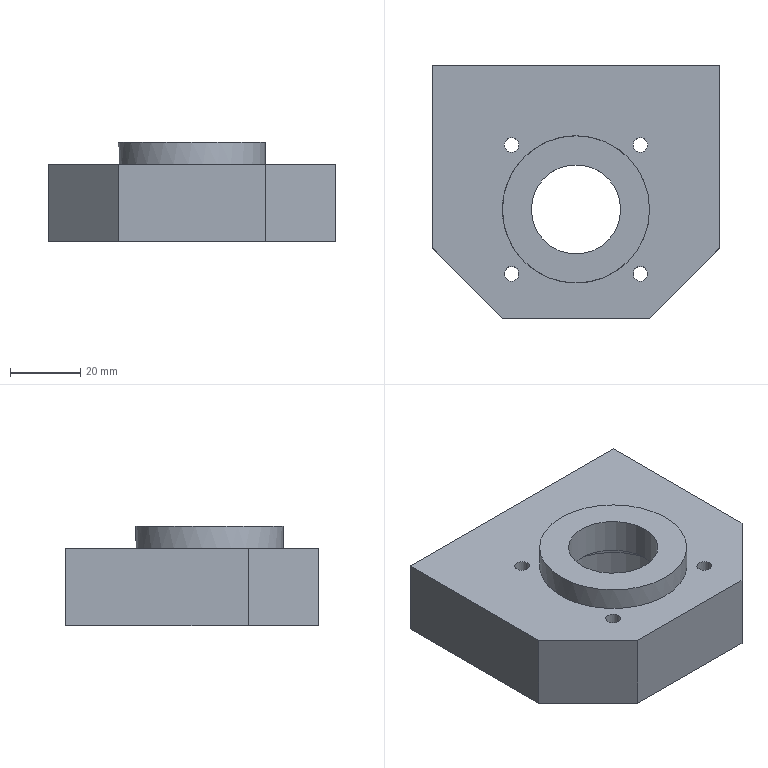Part | NX | features EXTRUDE 7, DATUM_CSYS 2, SKETCH 2, LINKED_FACE 1 | 1 solid | 23 faces | box 82 x 72 x 28.5 mm | volume 96953 mm3 | plane 13 | cylinder 10 | commonest cylinder face diameters 4.2 x4 8.5 x2 42 x2 25.5 x1 36 x1
STEP:
#1=CARTESIAN_POINT('',(-18.,0.,3.));
#2=VERTEX_POINT('',#1);
#3=CARTESIAN_POINT('',(0.,0.,3.));
#4=DIRECTION('',(0.,0.,1.));
#5=DIRECTION('',(-1.,0.,0.));
#6=AXIS2_PLACEMENT_3D('',#3,#4,#5);
#7=CIRCLE('',#6,18.);
#8=EDGE_CURVE('',#2,#2,#7,.T.);
#9=ORIENTED_EDGE('',*,*,#8,.F.);
#10=EDGE_LOOP('',(#9));
#11=FACE_BOUND('',#10,.T.);
#12=CARTESIAN_POINT('',(18.,0.,7.5));
#13=VERTEX_POINT('',#12);
#14=CARTESIAN_POINT('',(0.,0.,7.5));
#15=DIRECTION('',(0.,0.,-1.));
#16=DIRECTION('',(1.,0.,0.));
#17=AXIS2_PLACEMENT_3D('',#14,#15,#16);
#18=CIRCLE('',#17,18.);
#19=EDGE_CURVE('',#13,#13,#18,.T.);
#20=ORIENTED_EDGE('',*,*,#19,.F.);
#21=EDGE_LOOP('',(#20));
#22=FACE_BOUND('',#21,.T.);
#23=CARTESIAN_POINT('',(0.,0.,3.));
#24=DIRECTION('',(0.,0.,1.));
#25=DIRECTION('',(1.,0.,0.));
#26=AXIS2_PLACEMENT_3D('',#23,#24,#25);
#27=CYLINDRICAL_SURFACE('',#26,18.);
#28=ADVANCED_FACE('',(#11,#22),#27,.F.);
#29=CARTESIAN_POINT('',(21.,0.,-11.));
#30=VERTEX_POINT('',#29);
#31=CARTESIAN_POINT('',(0.,0.,-11.));
#32=DIRECTION('',(0.,0.,1.));
#33=DIRECTION('',(1.,0.,0.));
#34=AXIS2_PLACEMENT_3D('',#31,#32,#33);
#35=CIRCLE('',#34,21.);
#36=EDGE_CURVE('',#30,#30,#35,.F.);
#37=ORIENTED_EDGE('',*,*,#36,.T.);
#38=EDGE_LOOP('',(#37));
#39=FACE_BOUND('',#38,.T.);
#40=CARTESIAN_POINT('',(21.,0.,3.));
#41=VERTEX_POINT('',#40);
#42=CARTESIAN_POINT('',(0.,0.,3.));
#43=DIRECTION('',(0.,0.,1.));
#44=DIRECTION('',(1.,0.,0.));
#45=AXIS2_PLACEMENT_3D('',#42,#43,#44);
#46=CIRCLE('',#45,21.);
#47=EDGE_CURVE('',#41,#41,#46,.T.);
#48=ORIENTED_EDGE('',*,*,#47,.T.);
#49=EDGE_LOOP('',(#48));
#50=FACE_BOUND('',#49,.T.);
#51=CARTESIAN_POINT('',(0.,0.,9.));
#52=DIRECTION('',(0.,0.,-1.));
#53=DIRECTION('',(-1.,0.,0.));
#54=AXIS2_PLACEMENT_3D('',#51,#52,#53);
#55=CYLINDRICAL_SURFACE('',#54,21.);
#56=ADVANCED_FACE('',(#39,#50),#55,.F.);
#57=CARTESIAN_POINT('',(41.,-11.,-11.));
#58=VERTEX_POINT('',#57);
#59=CARTESIAN_POINT('',(41.,41.,-11.));
#60=VERTEX_POINT('',#59);
#61=CARTESIAN_POINT('',(41.,-11.,-11.));
#62=DIRECTION('',(0.,1.,0.));
#63=VECTOR('',#62,1000.);
#64=LINE('',#61,#63);
#65=EDGE_CURVE('',#58,#60,#64,.T.);
#66=ORIENTED_EDGE('',*,*,#65,.T.);
#67=CARTESIAN_POINT('',(41.,41.,11.));
#68=VERTEX_POINT('',#67);
#69=CARTESIAN_POINT('',(41.,41.,11.));
#70=DIRECTION('',(0.,0.,-1.));
#71=VECTOR('',#70,1000.);
#72=LINE('',#69,#71);
#73=EDGE_CURVE('',#68,#60,#72,.T.);
#74=ORIENTED_EDGE('',*,*,#73,.F.);
#75=CARTESIAN_POINT('',(41.,-11.,11.));
#76=VERTEX_POINT('',#75);
#77=CARTESIAN_POINT('',(41.,-11.,11.));
#78=DIRECTION('',(0.,1.,0.));
#79=VECTOR('',#78,1000.);
#80=LINE('',#77,#79);
#81=EDGE_CURVE('',#76,#68,#80,.T.);
#82=ORIENTED_EDGE('',*,*,#81,.F.);
#83=CARTESIAN_POINT('',(41.,-11.,11.));
#84=DIRECTION('',(0.,0.,-1.));
#85=VECTOR('',#84,1000.);
#86=LINE('',#83,#85);
#87=EDGE_CURVE('',#76,#58,#86,.T.);
#88=ORIENTED_EDGE('',*,*,#87,.T.);
#89=EDGE_LOOP('',(#66,#74,#82,#88));
#90=FACE_BOUND('',#89,.T.);
#91=CARTESIAN_POINT('',(41.,-11.,11.));
#92=DIRECTION('',(-1.,0.,0.));
#93=DIRECTION('',(0.,0.,1.));
#94=AXIS2_PLACEMENT_3D('',#91,#92,#93);
#95=PLANE('',#94);
#96=ADVANCED_FACE('',(#90),#95,.F.);
#97=CARTESIAN_POINT('',(30.,41.,-4.25));
#98=VERTEX_POINT('',#97);
#99=CARTESIAN_POINT('',(30.,41.,0.));
#100=DIRECTION('',(0.,-1.,0.));
#101=DIRECTION('',(0.,0.,-1.));
#102=AXIS2_PLACEMENT_3D('',#99,#100,#101);
#103=CIRCLE('',#102,4.25);
#104=EDGE_CURVE('',#98,#98,#103,.T.);
#105=ORIENTED_EDGE('',*,*,#104,.T.);
#106=EDGE_LOOP('',(#105));
#107=FACE_BOUND('',#106,.T.);
#108=CARTESIAN_POINT('',(-30.,41.,-4.25));
#109=VERTEX_POINT('',#108);
#110=CARTESIAN_POINT('',(-30.,41.,0.));
#111=DIRECTION('',(0.,-1.,0.));
#112=DIRECTION('',(0.,0.,-1.));
#113=AXIS2_PLACEMENT_3D('',#110,#111,#112);
#114=CIRCLE('',#113,4.25);
#115=EDGE_CURVE('',#109,#109,#114,.T.);
#116=ORIENTED_EDGE('',*,*,#115,.T.);
#117=EDGE_LOOP('',(#116));
#118=FACE_BOUND('',#117,.T.);
#119=CARTESIAN_POINT('',(-41.,41.,-11.));
#120=VERTEX_POINT('',#119);
#121=CARTESIAN_POINT('',(41.,41.,-11.));
#122=DIRECTION('',(-1.,0.,0.));
#123=VECTOR('',#122,1000.);
#124=LINE('',#121,#123);
#125=EDGE_CURVE('',#60,#120,#124,.T.);
#126=ORIENTED_EDGE('',*,*,#125,.T.);
#127=CARTESIAN_POINT('',(-41.,41.,11.));
#128=VERTEX_POINT('',#127);
#129=CARTESIAN_POINT('',(-41.,41.,11.));
#130=DIRECTION('',(0.,0.,-1.));
#131=VECTOR('',#130,1000.);
#132=LINE('',#129,#131);
#133=EDGE_CURVE('',#128,#120,#132,.T.);
#134=ORIENTED_EDGE('',*,*,#133,.F.);
#135=CARTESIAN_POINT('',(41.,41.,11.));
#136=DIRECTION('',(-1.,0.,0.));
#137=VECTOR('',#136,1000.);
#138=LINE('',#135,#137);
#139=EDGE_CURVE('',#68,#128,#138,.T.);
#140=ORIENTED_EDGE('',*,*,#139,.F.);
#141=ORIENTED_EDGE('',*,*,#73,.T.);
#142=EDGE_LOOP('',(#126,#134,#140,#141));
#143=FACE_BOUND('',#142,.T.);
#144=CARTESIAN_POINT('',(41.,41.,11.));
#145=DIRECTION('',(0.,-1.,0.));
#146=DIRECTION('',(0.,0.,-1.));
#147=AXIS2_PLACEMENT_3D('',#144,#145,#146);
#148=PLANE('',#147);
#149=ADVANCED_FACE('',(#107,#118,#143),#148,.F.);
#150=CARTESIAN_POINT('',(-41.,-11.,-11.));
#151=VERTEX_POINT('',#150);
#152=CARTESIAN_POINT('',(-41.,41.,-11.));
#153=DIRECTION('',(0.,-1.,0.));
#154=VECTOR('',#153,1000.);
#155=LINE('',#152,#154);
#156=EDGE_CURVE('',#120,#151,#155,.T.);
#157=ORIENTED_EDGE('',*,*,#156,.T.);
#158=CARTESIAN_POINT('',(-41.,-11.,11.));
#159=VERTEX_POINT('',#158);
#160=CARTESIAN_POINT('',(-41.,-11.,11.));
#161=DIRECTION('',(0.,0.,-1.));
#162=VECTOR('',#161,1000.);
#163=LINE('',#160,#162);
#164=EDGE_CURVE('',#159,#151,#163,.T.);
#165=ORIENTED_EDGE('',*,*,#164,.F.);
#166=CARTESIAN_POINT('',(-41.,41.,11.));
#167=DIRECTION('',(0.,-1.,0.));
#168=VECTOR('',#167,1000.);
#169=LINE('',#166,#168);
#170=EDGE_CURVE('',#128,#159,#169,.T.);
#171=ORIENTED_EDGE('',*,*,#170,.F.);
#172=ORIENTED_EDGE('',*,*,#133,.T.);
#173=EDGE_LOOP('',(#157,#165,#171,#172));
#174=FACE_BOUND('',#173,.T.);
#175=CARTESIAN_POINT('',(-41.,41.,11.));
#176=DIRECTION('',(1.,0.,0.));
#177=DIRECTION('',(0.,0.,-1.));
#178=AXIS2_PLACEMENT_3D('',#175,#176,#177);
#179=PLANE('',#178);
#180=ADVANCED_FACE('',(#174),#179,.F.);
#181=CARTESIAN_POINT('',(-21.,-31.,-11.));
#182=VERTEX_POINT('',#181);
#183=CARTESIAN_POINT('',(-41.,-11.,-11.));
#184=DIRECTION('',(0.7071,-0.7071,0.));
#185=VECTOR('',#184,1000.);
#186=LINE('',#183,#185);
#187=EDGE_CURVE('',#151,#182,#186,.T.);
#188=ORIENTED_EDGE('',*,*,#187,.T.);
#189=CARTESIAN_POINT('',(-21.,-31.,11.));
#190=VERTEX_POINT('',#189);
#191=CARTESIAN_POINT('',(-21.,-31.,11.));
#192=DIRECTION('',(0.,0.,-1.));
#193=VECTOR('',#192,1000.);
#194=LINE('',#191,#193);
#195=EDGE_CURVE('',#190,#182,#194,.T.);
#196=ORIENTED_EDGE('',*,*,#195,.F.);
#197=CARTESIAN_POINT('',(-41.,-11.,11.));
#198=DIRECTION('',(0.7071,-0.7071,0.));
#199=VECTOR('',#198,1000.);
#200=LINE('',#197,#199);
#201=EDGE_CURVE('',#159,#190,#200,.T.);
#202=ORIENTED_EDGE('',*,*,#201,.F.);
#203=ORIENTED_EDGE('',*,*,#164,.T.);
#204=EDGE_LOOP('',(#188,#196,#202,#203));
#205=FACE_BOUND('',#204,.T.);
#206=CARTESIAN_POINT('',(-41.,-11.,11.));
#207=DIRECTION('',(0.7071,0.7071,0.));
#208=DIRECTION('',(-0.7071,0.7071,0.));
#209=AXIS2_PLACEMENT_3D('',#206,#207,#208);
#210=PLANE('',#209);
#211=ADVANCED_FACE('',(#205),#210,.F.);
#212=CARTESIAN_POINT('',(21.,-31.,-11.));
#213=VERTEX_POINT('',#212);
#214=CARTESIAN_POINT('',(-21.,-31.,-11.));
#215=DIRECTION('',(1.,0.,0.));
#216=VECTOR('',#215,1000.);
#217=LINE('',#214,#216);
#218=EDGE_CURVE('',#182,#213,#217,.T.);
#219=ORIENTED_EDGE('',*,*,#218,.T.);
#220=CARTESIAN_POINT('',(21.,-31.,11.));
#221=VERTEX_POINT('',#220);
#222=CARTESIAN_POINT('',(21.,-31.,11.));
#223=DIRECTION('',(0.,0.,-1.));
#224=VECTOR('',#223,1000.);
#225=LINE('',#222,#224);
#226=EDGE_CURVE('',#221,#213,#225,.T.);
#227=ORIENTED_EDGE('',*,*,#226,.F.);
#228=CARTESIAN_POINT('',(-21.,-31.,11.));
#229=DIRECTION('',(1.,0.,0.));
#230=VECTOR('',#229,1000.);
#231=LINE('',#228,#230);
#232=EDGE_CURVE('',#190,#221,#231,.T.);
#233=ORIENTED_EDGE('',*,*,#232,.F.);
#234=ORIENTED_EDGE('',*,*,#195,.T.);
#235=EDGE_LOOP('',(#219,#227,#233,#234));
#236=FACE_BOUND('',#235,.T.);
#237=CARTESIAN_POINT('',(-21.,-31.,11.));
#238=DIRECTION('',(0.,1.,0.));
#239=DIRECTION('',(0.,0.,1.));
#240=AXIS2_PLACEMENT_3D('',#237,#238,#239);
#241=PLANE('',#240);
#242=ADVANCED_FACE('',(#236),#241,.F.);
#243=CARTESIAN_POINT('',(21.,-31.,-11.));
#244=DIRECTION('',(0.7071,0.7071,0.));
#245=VECTOR('',#244,1000.);
#246=LINE('',#243,#245);
#247=EDGE_CURVE('',#213,#58,#246,.T.);
#248=ORIENTED_EDGE('',*,*,#247,.T.);
#249=ORIENTED_EDGE('',*,*,#87,.F.);
#250=CARTESIAN_POINT('',(21.,-31.,11.));
#251=DIRECTION('',(0.7071,0.7071,0.));
#252=VECTOR('',#251,1000.);
#253=LINE('',#250,#252);
#254=EDGE_CURVE('',#221,#76,#253,.T.);
#255=ORIENTED_EDGE('',*,*,#254,.F.);
#256=ORIENTED_EDGE('',*,*,#226,.T.);
#257=EDGE_LOOP('',(#248,#249,#255,#256));
#258=FACE_BOUND('',#257,.T.);
#259=CARTESIAN_POINT('',(21.,-31.,11.));
#260=DIRECTION('',(-0.7071,0.7071,0.));
#261=DIRECTION('',(-0.7071,-0.7071,0.));
#262=AXIS2_PLACEMENT_3D('',#259,#260,#261);
#263=PLANE('',#262);
#264=ADVANCED_FACE('',(#258),#263,.F.);
#265=CARTESIAN_POINT('',(21.,0.,11.));
#266=VERTEX_POINT('',#265);
#267=CARTESIAN_POINT('',(0.,0.,11.));
#268=DIRECTION('',(0.,0.,1.));
#269=DIRECTION('',(1.,0.,0.));
#270=AXIS2_PLACEMENT_3D('',#267,#268,#269);
#271=CIRCLE('',#270,21.);
#272=EDGE_CURVE('',#266,#266,#271,.T.);
#273=ORIENTED_EDGE('',*,*,#272,.F.);
#274=EDGE_LOOP('',(#273));
#275=FACE_BOUND('',#274,.T.);
#276=CARTESIAN_POINT('',(20.485,-18.385,11.));
#277=VERTEX_POINT('',#276);
#278=CARTESIAN_POINT('',(18.385,-18.385,11.));
#279=DIRECTION('',(0.,0.,1.));
#280=DIRECTION('',(1.,0.,0.));
#281=AXIS2_PLACEMENT_3D('',#278,#279,#280);
#282=CIRCLE('',#281,2.1);
#283=EDGE_CURVE('',#277,#277,#282,.T.);
#284=ORIENTED_EDGE('',*,*,#283,.F.);
#285=EDGE_LOOP('',(#284));
#286=FACE_BOUND('',#285,.T.);
#287=CARTESIAN_POINT('',(-16.285,18.385,11.));
#288=VERTEX_POINT('',#287);
#289=CARTESIAN_POINT('',(-18.385,18.385,11.));
#290=DIRECTION('',(0.,0.,1.));
#291=DIRECTION('',(1.,0.,0.));
#292=AXIS2_PLACEMENT_3D('',#289,#290,#291);
#293=CIRCLE('',#292,2.1);
#294=EDGE_CURVE('',#288,#288,#293,.T.);
#295=ORIENTED_EDGE('',*,*,#294,.F.);
#296=EDGE_LOOP('',(#295));
#297=FACE_BOUND('',#296,.T.);
#298=CARTESIAN_POINT('',(-16.285,-18.385,11.));
#299=VERTEX_POINT('',#298);
#300=CARTESIAN_POINT('',(-18.385,-18.385,11.));
#301=DIRECTION('',(0.,0.,1.));
#302=DIRECTION('',(1.,0.,0.));
#303=AXIS2_PLACEMENT_3D('',#300,#301,#302);
#304=CIRCLE('',#303,2.1);
#305=EDGE_CURVE('',#299,#299,#304,.T.);
#306=ORIENTED_EDGE('',*,*,#305,.F.);
#307=EDGE_LOOP('',(#306));
#308=FACE_BOUND('',#307,.T.);
#309=CARTESIAN_POINT('',(20.485,18.385,11.));
#310=VERTEX_POINT('',#309);
#311=CARTESIAN_POINT('',(18.385,18.385,11.));
#312=DIRECTION('',(0.,0.,1.));
#313=DIRECTION('',(1.,0.,0.));
#314=AXIS2_PLACEMENT_3D('',#311,#312,#313);
#315=CIRCLE('',#314,2.1);
#316=EDGE_CURVE('',#310,#310,#315,.T.);
#317=ORIENTED_EDGE('',*,*,#316,.F.);
#318=EDGE_LOOP('',(#317));
#319=FACE_BOUND('',#318,.T.);
#320=ORIENTED_EDGE('',*,*,#81,.T.);
#321=ORIENTED_EDGE('',*,*,#139,.T.);
#322=ORIENTED_EDGE('',*,*,#170,.T.);
#323=ORIENTED_EDGE('',*,*,#201,.T.);
#324=ORIENTED_EDGE('',*,*,#232,.T.);
#325=ORIENTED_EDGE('',*,*,#254,.T.);
#326=EDGE_LOOP('',(#320,#321,#322,#323,#324,#325));
#327=FACE_BOUND('',#326,.T.);
#328=CARTESIAN_POINT('',(0.,0.,11.));
#329=DIRECTION('',(0.,0.,1.));
#330=DIRECTION('',(1.,0.,0.));
#331=AXIS2_PLACEMENT_3D('',#328,#329,#330);
#332=PLANE('',#331);
#333=ADVANCED_FACE('',(#275,#286,#297,#308,#319,#327),#332,.T.);
#334=CARTESIAN_POINT('',(20.485,-18.385,-11.));
#335=VERTEX_POINT('',#334);
#336=CARTESIAN_POINT('',(18.385,-18.385,-11.));
#337=DIRECTION('',(0.,0.,1.));
#338=DIRECTION('',(1.,0.,0.));
#339=AXIS2_PLACEMENT_3D('',#336,#337,#338);
#340=CIRCLE('',#339,2.1);
#341=EDGE_CURVE('',#335,#335,#340,.T.);
#342=ORIENTED_EDGE('',*,*,#341,.T.);
#343=EDGE_LOOP('',(#342));
#344=FACE_BOUND('',#343,.T.);
#345=CARTESIAN_POINT('',(-16.285,18.385,-11.));
#346=VERTEX_POINT('',#345);
#347=CARTESIAN_POINT('',(-18.385,18.385,-11.));
#348=DIRECTION('',(0.,0.,1.));
#349=DIRECTION('',(1.,0.,0.));
#350=AXIS2_PLACEMENT_3D('',#347,#348,#349);
#351=CIRCLE('',#350,2.1);
#352=EDGE_CURVE('',#346,#346,#351,.T.);
#353=ORIENTED_EDGE('',*,*,#352,.T.);
#354=EDGE_LOOP('',(#353));
#355=FACE_BOUND('',#354,.T.);
#356=CARTESIAN_POINT('',(-16.285,-18.385,-11.));
#357=VERTEX_POINT('',#356);
#358=CARTESIAN_POINT('',(-18.385,-18.385,-11.));
#359=DIRECTION('',(0.,0.,1.));
#360=DIRECTION('',(1.,0.,0.));
#361=AXIS2_PLACEMENT_3D('',#358,#359,#360);
#362=CIRCLE('',#361,2.1);
#363=EDGE_CURVE('',#357,#357,#362,.T.);
#364=ORIENTED_EDGE('',*,*,#363,.T.);
#365=EDGE_LOOP('',(#364));
#366=FACE_BOUND('',#365,.T.);
#367=CARTESIAN_POINT('',(20.485,18.385,-11.));
#368=VERTEX_POINT('',#367);
#369=CARTESIAN_POINT('',(18.385,18.385,-11.));
#370=DIRECTION('',(0.,0.,1.));
#371=DIRECTION('',(1.,0.,0.));
#372=AXIS2_PLACEMENT_3D('',#369,#370,#371);
#373=CIRCLE('',#372,2.1);
#374=EDGE_CURVE('',#368,#368,#373,.T.);
#375=ORIENTED_EDGE('',*,*,#374,.T.);
#376=EDGE_LOOP('',(#375));
#377=FACE_BOUND('',#376,.T.);
#378=ORIENTED_EDGE('',*,*,#36,.F.);
#379=EDGE_LOOP('',(#378));
#380=FACE_BOUND('',#379,.T.);
#381=ORIENTED_EDGE('',*,*,#65,.F.);
#382=ORIENTED_EDGE('',*,*,#247,.F.);
#383=ORIENTED_EDGE('',*,*,#218,.F.);
#384=ORIENTED_EDGE('',*,*,#187,.F.);
#385=ORIENTED_EDGE('',*,*,#156,.F.);
#386=ORIENTED_EDGE('',*,*,#125,.F.);
#387=EDGE_LOOP('',(#381,#382,#383,#384,#385,#386));
#388=FACE_BOUND('',#387,.T.);
#389=CARTESIAN_POINT('',(0.,0.,-11.));
#390=DIRECTION('',(0.,0.,1.));
#391=DIRECTION('',(1.,0.,0.));
#392=AXIS2_PLACEMENT_3D('',#389,#390,#391);
#393=PLANE('',#392);
#394=ADVANCED_FACE('',(#344,#355,#366,#377,#380,#388),#393,.F.);
#395=CARTESIAN_POINT('',(-30.,16.,4.25));
#396=VERTEX_POINT('',#395);
#397=CARTESIAN_POINT('',(-30.,16.,0.));
#398=DIRECTION('',(0.,1.,0.));
#399=DIRECTION('',(0.,0.,1.));
#400=AXIS2_PLACEMENT_3D('',#397,#398,#399);
#401=CIRCLE('',#400,4.25);
#402=EDGE_CURVE('',#396,#396,#401,.F.);
#403=ORIENTED_EDGE('',*,*,#402,.T.);
#404=EDGE_LOOP('',(#403));
#405=FACE_BOUND('',#404,.T.);
#406=ORIENTED_EDGE('',*,*,#115,.F.);
#407=EDGE_LOOP('',(#406));
#408=FACE_BOUND('',#407,.T.);
#409=CARTESIAN_POINT('',(-30.,16.,0.));
#410=DIRECTION('',(0.,1.,0.));
#411=DIRECTION('',(0.,0.,1.));
#412=AXIS2_PLACEMENT_3D('',#409,#410,#411);
#413=CYLINDRICAL_SURFACE('',#412,4.25);
#414=ADVANCED_FACE('',(#405,#408),#413,.F.);
#415=ORIENTED_EDGE('',*,*,#402,.F.);
#416=EDGE_LOOP('',(#415));
#417=FACE_BOUND('',#416,.T.);
#418=CARTESIAN_POINT('',(-30.,16.,0.));
#419=DIRECTION('',(0.,1.,0.));
#420=DIRECTION('',(0.,0.,1.));
#421=AXIS2_PLACEMENT_3D('',#418,#419,#420);
#422=PLANE('',#421);
#423=ADVANCED_FACE('',(#417),#422,.T.);
#424=CARTESIAN_POINT('',(30.,16.,4.25));
#425=VERTEX_POINT('',#424);
#426=CARTESIAN_POINT('',(30.,16.,0.));
#427=DIRECTION('',(0.,1.,0.));
#428=DIRECTION('',(0.,0.,1.));
#429=AXIS2_PLACEMENT_3D('',#426,#427,#428);
#430=CIRCLE('',#429,4.25);
#431=EDGE_CURVE('',#425,#425,#430,.F.);
#432=ORIENTED_EDGE('',*,*,#431,.T.);
#433=EDGE_LOOP('',(#432));
#434=FACE_BOUND('',#433,.T.);
#435=ORIENTED_EDGE('',*,*,#104,.F.);
#436=EDGE_LOOP('',(#435));
#437=FACE_BOUND('',#436,.T.);
#438=CARTESIAN_POINT('',(30.,16.,0.));
#439=DIRECTION('',(0.,1.,0.));
#440=DIRECTION('',(0.,0.,1.));
#441=AXIS2_PLACEMENT_3D('',#438,#439,#440);
#442=CYLINDRICAL_SURFACE('',#441,4.25);
#443=ADVANCED_FACE('',(#434,#437),#442,.F.);
#444=ORIENTED_EDGE('',*,*,#431,.F.);
#445=EDGE_LOOP('',(#444));
#446=FACE_BOUND('',#445,.T.);
#447=CARTESIAN_POINT('',(30.,16.,0.));
#448=DIRECTION('',(0.,1.,0.));
#449=DIRECTION('',(0.,0.,1.));
#450=AXIS2_PLACEMENT_3D('',#447,#448,#449);
#451=PLANE('',#450);
#452=ADVANCED_FACE('',(#446),#451,.T.);
#453=ORIENTED_EDGE('',*,*,#316,.T.);
#454=EDGE_LOOP('',(#453));
#455=FACE_BOUND('',#454,.T.);
#456=ORIENTED_EDGE('',*,*,#374,.F.);
#457=EDGE_LOOP('',(#456));
#458=FACE_BOUND('',#457,.T.);
#459=CARTESIAN_POINT('',(18.385,18.385,-27.5));
#460=DIRECTION('',(0.,0.,1.));
#461=DIRECTION('',(1.,0.,0.));
#462=AXIS2_PLACEMENT_3D('',#459,#460,#461);
#463=CYLINDRICAL_SURFACE('',#462,2.1);
#464=ADVANCED_FACE('',(#455,#458),#463,.F.);
#465=ORIENTED_EDGE('',*,*,#305,.T.);
#466=EDGE_LOOP('',(#465));
#467=FACE_BOUND('',#466,.T.);
#468=ORIENTED_EDGE('',*,*,#363,.F.);
#469=EDGE_LOOP('',(#468));
#470=FACE_BOUND('',#469,.T.);
#471=CARTESIAN_POINT('',(-18.385,-18.385,-27.5));
#472=DIRECTION('',(0.,0.,1.));
#473=DIRECTION('',(1.,0.,0.));
#474=AXIS2_PLACEMENT_3D('',#471,#472,#473);
#475=CYLINDRICAL_SURFACE('',#474,2.1);
#476=ADVANCED_FACE('',(#467,#470),#475,.F.);
#477=ORIENTED_EDGE('',*,*,#294,.T.);
#478=EDGE_LOOP('',(#477));
#479=FACE_BOUND('',#478,.T.);
#480=ORIENTED_EDGE('',*,*,#352,.F.);
#481=EDGE_LOOP('',(#480));
#482=FACE_BOUND('',#481,.T.);
#483=CARTESIAN_POINT('',(-18.385,18.385,-27.5));
#484=DIRECTION('',(0.,0.,1.));
#485=DIRECTION('',(1.,0.,0.));
#486=AXIS2_PLACEMENT_3D('',#483,#484,#485);
#487=CYLINDRICAL_SURFACE('',#486,2.1);
#488=ADVANCED_FACE('',(#479,#482),#487,.F.);
#489=ORIENTED_EDGE('',*,*,#283,.T.);
#490=EDGE_LOOP('',(#489));
#491=FACE_BOUND('',#490,.T.);
#492=ORIENTED_EDGE('',*,*,#341,.F.);
#493=EDGE_LOOP('',(#492));
#494=FACE_BOUND('',#493,.T.);
#495=CARTESIAN_POINT('',(18.385,-18.385,-27.5));
#496=DIRECTION('',(0.,0.,1.));
#497=DIRECTION('',(1.,0.,0.));
#498=AXIS2_PLACEMENT_3D('',#495,#496,#497);
#499=CYLINDRICAL_SURFACE('',#498,2.1);
#500=ADVANCED_FACE('',(#491,#494),#499,.F.);
#501=ORIENTED_EDGE('',*,*,#47,.F.);
#502=EDGE_LOOP('',(#501));
#503=FACE_BOUND('',#502,.T.);
#504=ORIENTED_EDGE('',*,*,#8,.T.);
#505=EDGE_LOOP('',(#504));
#506=FACE_BOUND('',#505,.T.);
#507=CARTESIAN_POINT('',(0.,0.,3.));
#508=DIRECTION('',(0.,0.,1.));
#509=DIRECTION('',(1.,0.,0.));
#510=AXIS2_PLACEMENT_3D('',#507,#508,#509);
#511=PLANE('',#510);
#512=ADVANCED_FACE('',(#503,#506),#511,.F.);
#513=ORIENTED_EDGE('',*,*,#272,.T.);
#514=EDGE_LOOP('',(#513));
#515=FACE_BOUND('',#514,.T.);
#516=CARTESIAN_POINT('',(-21.,0.,17.5));
#517=VERTEX_POINT('',#516);
#518=CARTESIAN_POINT('',(0.,0.,17.5));
#519=DIRECTION('',(0.,0.,1.));
#520=DIRECTION('',(-1.,0.,0.));
#521=AXIS2_PLACEMENT_3D('',#518,#519,#520);
#522=CIRCLE('',#521,21.);
#523=EDGE_CURVE('',#517,#517,#522,.T.);
#524=ORIENTED_EDGE('',*,*,#523,.F.);
#525=EDGE_LOOP('',(#524));
#526=FACE_BOUND('',#525,.T.);
#527=CARTESIAN_POINT('',(0.,0.,3.));
#528=DIRECTION('',(0.,0.,1.));
#529=DIRECTION('',(1.,0.,0.));
#530=AXIS2_PLACEMENT_3D('',#527,#528,#529);
#531=CYLINDRICAL_SURFACE('',#530,21.);
#532=ADVANCED_FACE('',(#515,#526),#531,.T.);
#533=ORIENTED_EDGE('',*,*,#523,.T.);
#534=EDGE_LOOP('',(#533));
#535=FACE_BOUND('',#534,.T.);
#536=CARTESIAN_POINT('',(-12.75,0.,17.5));
#537=VERTEX_POINT('',#536);
#538=CARTESIAN_POINT('',(0.,0.,17.5));
#539=DIRECTION('',(0.,0.,1.));
#540=DIRECTION('',(-1.,0.,0.));
#541=AXIS2_PLACEMENT_3D('',#538,#539,#540);
#542=CIRCLE('',#541,12.75);
#543=EDGE_CURVE('',#537,#537,#542,.T.);
#544=ORIENTED_EDGE('',*,*,#543,.F.);
#545=EDGE_LOOP('',(#544));
#546=FACE_BOUND('',#545,.T.);
#547=CARTESIAN_POINT('',(0.,0.,17.5));
#548=DIRECTION('',(0.,0.,1.));
#549=DIRECTION('',(1.,0.,0.));
#550=AXIS2_PLACEMENT_3D('',#547,#548,#549);
#551=PLANE('',#550);
#552=ADVANCED_FACE('',(#535,#546),#551,.T.);
#553=ORIENTED_EDGE('',*,*,#543,.T.);
#554=EDGE_LOOP('',(#553));
#555=FACE_BOUND('',#554,.T.);
#556=CARTESIAN_POINT('',(12.75,0.,7.5));
#557=VERTEX_POINT('',#556);
#558=CARTESIAN_POINT('',(0.,0.,7.5));
#559=DIRECTION('',(0.,0.,1.));
#560=DIRECTION('',(1.,0.,0.));
#561=AXIS2_PLACEMENT_3D('',#558,#559,#560);
#562=CIRCLE('',#561,12.75);
#563=EDGE_CURVE('',#557,#557,#562,.T.);
#564=ORIENTED_EDGE('',*,*,#563,.F.);
#565=EDGE_LOOP('',(#564));
#566=FACE_BOUND('',#565,.T.);
#567=CARTESIAN_POINT('',(0.,0.,43.5));
#568=DIRECTION('',(0.,0.,-1.));
#569=DIRECTION('',(-1.,0.,0.));
#570=AXIS2_PLACEMENT_3D('',#567,#568,#569);
#571=CYLINDRICAL_SURFACE('',#570,12.75);
#572=ADVANCED_FACE('',(#555,#566),#571,.F.);
#573=ORIENTED_EDGE('',*,*,#19,.T.);
#574=EDGE_LOOP('',(#573));
#575=FACE_BOUND('',#574,.T.);
#576=ORIENTED_EDGE('',*,*,#563,.T.);
#577=EDGE_LOOP('',(#576));
#578=FACE_BOUND('',#577,.T.);
#579=CARTESIAN_POINT('',(0.,0.,7.5));
#580=DIRECTION('',(0.,0.,-1.));
#581=DIRECTION('',(-1.,0.,0.));
#582=AXIS2_PLACEMENT_3D('',#579,#580,#581);
#583=PLANE('',#582);
#584=ADVANCED_FACE('',(#575,#578),#583,.T.);
#585=CLOSED_SHELL('',(#28,#56,#96,#149,#180,#211,#242,#264,#333,#394,#414,#423,#443,#452,#464,#476,#488,#500,#512,#532,#552,#572,#584));
#586=MANIFOLD_SOLID_BREP('',#585);
#587=(LENGTH_UNIT()NAMED_UNIT(*)SI_UNIT(.MILLI.,.METRE.));
#588=UNCERTAINTY_MEASURE_WITH_UNIT(LENGTH_MEASURE(0.00001),#587,'','');
#589=(NAMED_UNIT(*)PLANE_ANGLE_UNIT()SI_UNIT($,.RADIAN.));
#590=(NAMED_UNIT(*)SI_UNIT($,.STERADIAN.)SOLID_ANGLE_UNIT());
#591=(GEOMETRIC_REPRESENTATION_CONTEXT(3)GLOBAL_UNCERTAINTY_ASSIGNED_CONTEXT((#588))GLOBAL_UNIT_ASSIGNED_CONTEXT((#587,#589,#590))REPRESENTATION_CONTEXT('',''));
#592=ADVANCED_BREP_SHAPE_REPRESENTATION('',(#586),#591);